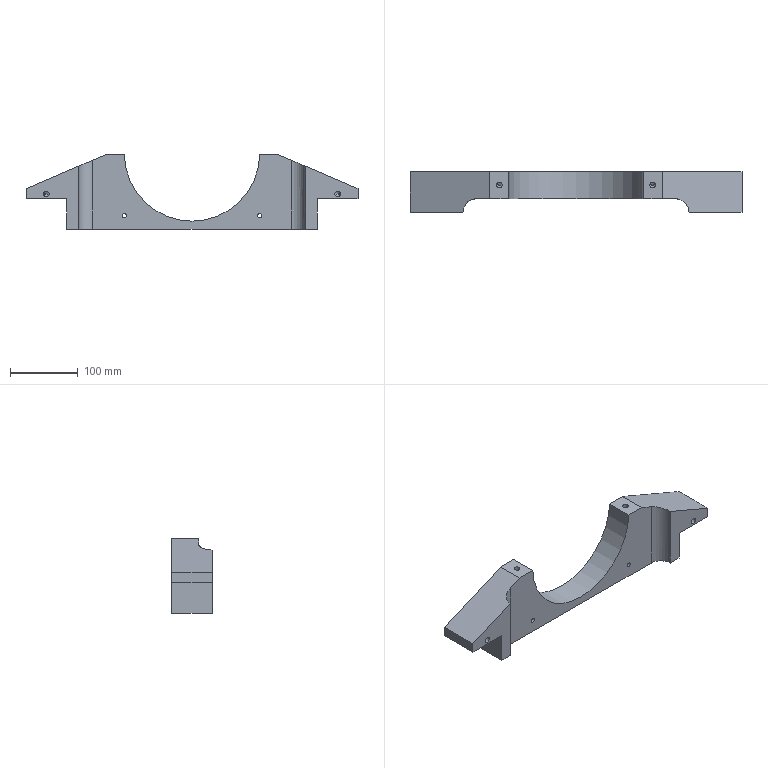Part | NX | features BREP 1 | 1 solid | 44 faces | box 490 x 60 x 110 mm | volume 1231742 mm3 | cylinder 19 | plane 17 | cone 8 | commonest cylinder face diameters 8.376 x8 6.4 x4 11.2 x4 40 x2 200 x1
STEP:
#1=CARTESIAN_POINT('',(185.,20.,-111.215));
#2=VERTEX_POINT('',#1);
#3=CARTESIAN_POINT('',(185.,20.,-66.215));
#4=VERTEX_POINT('',#3);
#5=CARTESIAN_POINT('',(185.,20.,-111.215));
#6=DIRECTION('',(0.,0.,1.));
#7=VECTOR('',#6,1000.);
#8=LINE('',#5,#7);
#9=EDGE_CURVE('',#2,#4,#8,.T.);
#10=ORIENTED_EDGE('',*,*,#9,.T.);
#11=CARTESIAN_POINT('',(185.,-40.,-66.215));
#12=VERTEX_POINT('',#11);
#13=CARTESIAN_POINT('',(185.,-40.,-66.215));
#14=DIRECTION('',(0.,1.,0.));
#15=VECTOR('',#14,1000.);
#16=LINE('',#13,#15);
#17=EDGE_CURVE('',#12,#4,#16,.T.);
#18=ORIENTED_EDGE('',*,*,#17,.F.);
#19=CARTESIAN_POINT('',(185.,-40.,-111.215));
#20=VERTEX_POINT('',#19);
#21=CARTESIAN_POINT('',(185.,-40.,-66.215));
#22=DIRECTION('',(0.,0.,-1.));
#23=VECTOR('',#22,1000.);
#24=LINE('',#21,#23);
#25=EDGE_CURVE('',#12,#20,#24,.T.);
#26=ORIENTED_EDGE('',*,*,#25,.T.);
#27=CARTESIAN_POINT('',(185.,-40.,-111.215));
#28=DIRECTION('',(0.,1.,0.));
#29=VECTOR('',#28,1000.);
#30=LINE('',#27,#29);
#31=EDGE_CURVE('',#20,#2,#30,.T.);
#32=ORIENTED_EDGE('',*,*,#31,.T.);
#33=EDGE_LOOP('',(#10,#18,#26,#32));
#34=FACE_BOUND('',#33,.T.);
#35=CARTESIAN_POINT('',(185.,0.,-121.215));
#36=DIRECTION('',(-1.,0.,0.));
#37=DIRECTION('',(0.,0.,1.));
#38=AXIS2_PLACEMENT_3D('',#35,#36,#37);
#39=PLANE('',#38);
#40=ADVANCED_FACE('',(#34),#39,.F.);
#41=CARTESIAN_POINT('',(-146.78,-20.,-111.215));
#42=VERTEX_POINT('',#41);
#43=CARTESIAN_POINT('',(-166.78,-40.,-111.215));
#44=VERTEX_POINT('',#43);
#45=CARTESIAN_POINT('',(-146.78,-40.,-111.215));
#46=DIRECTION('',(0.,0.,1.));
#47=DIRECTION('',(0.,1.,0.));
#48=AXIS2_PLACEMENT_3D('',#45,#46,#47);
#49=CIRCLE('',#48,20.);
#50=EDGE_CURVE('',#42,#44,#49,.T.);
#51=ORIENTED_EDGE('',*,*,#50,.T.);
#52=CARTESIAN_POINT('',(-185.,-40.,-111.215));
#53=VERTEX_POINT('',#52);
#54=CARTESIAN_POINT('',(-166.78,-40.,-111.215));
#55=DIRECTION('',(-1.,0.,0.));
#56=VECTOR('',#55,1000.);
#57=LINE('',#54,#56);
#58=EDGE_CURVE('',#44,#53,#57,.T.);
#59=ORIENTED_EDGE('',*,*,#58,.T.);
#60=CARTESIAN_POINT('',(-185.,20.,-111.215));
#61=VERTEX_POINT('',#60);
#62=CARTESIAN_POINT('',(-185.,-40.,-111.215));
#63=DIRECTION('',(0.,1.,0.));
#64=VECTOR('',#63,1000.);
#65=LINE('',#62,#64);
#66=EDGE_CURVE('',#53,#61,#65,.T.);
#67=ORIENTED_EDGE('',*,*,#66,.T.);
#68=CARTESIAN_POINT('',(185.,20.,-111.215));
#69=DIRECTION('',(-1.,0.,0.));
#70=VECTOR('',#69,1000.);
#71=LINE('',#68,#70);
#72=EDGE_CURVE('',#2,#61,#71,.T.);
#73=ORIENTED_EDGE('',*,*,#72,.F.);
#74=ORIENTED_EDGE('',*,*,#31,.F.);
#75=CARTESIAN_POINT('',(166.78,-40.,-111.215));
#76=VERTEX_POINT('',#75);
#77=CARTESIAN_POINT('',(166.78,-40.,-111.215));
#78=DIRECTION('',(1.,0.,0.));
#79=VECTOR('',#78,1000.);
#80=LINE('',#77,#79);
#81=EDGE_CURVE('',#76,#20,#80,.T.);
#82=ORIENTED_EDGE('',*,*,#81,.F.);
#83=CARTESIAN_POINT('',(146.78,-20.,-111.215));
#84=VERTEX_POINT('',#83);
#85=CARTESIAN_POINT('',(146.78,-40.,-111.215));
#86=DIRECTION('',(0.,0.,1.));
#87=DIRECTION('',(1.,0.,0.));
#88=AXIS2_PLACEMENT_3D('',#85,#86,#87);
#89=CIRCLE('',#88,20.);
#90=EDGE_CURVE('',#76,#84,#89,.T.);
#91=ORIENTED_EDGE('',*,*,#90,.T.);
#92=CARTESIAN_POINT('',(-146.78,-20.,-111.215));
#93=DIRECTION('',(1.,0.,0.));
#94=VECTOR('',#93,1000.);
#95=LINE('',#92,#94);
#96=EDGE_CURVE('',#42,#84,#95,.T.);
#97=ORIENTED_EDGE('',*,*,#96,.F.);
#98=EDGE_LOOP('',(#51,#59,#67,#73,#74,#82,#91,#97));
#99=FACE_BOUND('',#98,.T.);
#100=CARTESIAN_POINT('',(0.,0.,-111.215));
#101=DIRECTION('',(0.,0.,-1.));
#102=DIRECTION('',(0.,-1.,0.));
#103=AXIS2_PLACEMENT_3D('',#100,#101,#102);
#104=PLANE('',#103);
#105=ADVANCED_FACE('',(#99),#104,.T.);
#106=CARTESIAN_POINT('',(146.78,-20.,-9.42));
#107=VERTEX_POINT('',#106);
#108=CARTESIAN_POINT('',(146.78,-20.,-9.42));
#109=DIRECTION('',(0.,0.,-1.));
#110=VECTOR('',#109,1000.);
#111=LINE('',#108,#110);
#112=EDGE_CURVE('',#107,#84,#111,.T.);
#113=ORIENTED_EDGE('',*,*,#112,.F.);
#114=CARTESIAN_POINT('',(127.5,-20.,-1.215));
#115=VERTEX_POINT('',#114);
#116=CARTESIAN_POINT('',(146.78,-20.,-9.42));
#117=DIRECTION('',(-0.9202,0.,0.3916));
#118=VECTOR('',#117,1000.);
#119=LINE('',#116,#118);
#120=EDGE_CURVE('',#107,#115,#119,.T.);
#121=ORIENTED_EDGE('',*,*,#120,.T.);
#122=CARTESIAN_POINT('',(99.98,-20.,-1.215));
#123=VERTEX_POINT('',#122);
#124=CARTESIAN_POINT('',(127.5,-20.,-1.215));
#125=DIRECTION('',(-1.,0.,0.));
#126=VECTOR('',#125,1000.);
#127=LINE('',#124,#126);
#128=EDGE_CURVE('',#115,#123,#127,.T.);
#129=ORIENTED_EDGE('',*,*,#128,.T.);
#130=CARTESIAN_POINT('',(-99.98,-20.,-1.215));
#131=VERTEX_POINT('',#130);
#132=CARTESIAN_POINT('',(0.,-20.,0.7847));
#133=DIRECTION('',(0.,1.,0.));
#134=DIRECTION('',(0.9998,0.,-0.02));
#135=AXIS2_PLACEMENT_3D('',#132,#133,#134);
#136=CIRCLE('',#135,100.);
#137=EDGE_CURVE('',#123,#131,#136,.T.);
#138=ORIENTED_EDGE('',*,*,#137,.T.);
#139=CARTESIAN_POINT('',(-127.5,-20.,-1.215));
#140=VERTEX_POINT('',#139);
#141=CARTESIAN_POINT('',(-99.98,-20.,-1.215));
#142=DIRECTION('',(-1.,0.,0.));
#143=VECTOR('',#142,1000.);
#144=LINE('',#141,#143);
#145=EDGE_CURVE('',#131,#140,#144,.T.);
#146=ORIENTED_EDGE('',*,*,#145,.T.);
#147=CARTESIAN_POINT('',(-146.78,-20.,-9.42));
#148=VERTEX_POINT('',#147);
#149=CARTESIAN_POINT('',(-127.5,-20.,-1.215));
#150=DIRECTION('',(-0.9202,0.,-0.3916));
#151=VECTOR('',#150,1000.);
#152=LINE('',#149,#151);
#153=EDGE_CURVE('',#140,#148,#152,.T.);
#154=ORIENTED_EDGE('',*,*,#153,.T.);
#155=CARTESIAN_POINT('',(-146.78,-20.,-111.215));
#156=DIRECTION('',(0.,0.,1.));
#157=VECTOR('',#156,1000.);
#158=LINE('',#155,#157);
#159=EDGE_CURVE('',#42,#148,#158,.T.);
#160=ORIENTED_EDGE('',*,*,#159,.F.);
#161=ORIENTED_EDGE('',*,*,#96,.T.);
#162=EDGE_LOOP('',(#113,#121,#129,#138,#146,#154,#160,#161));
#163=FACE_BOUND('',#162,.T.);
#164=CARTESIAN_POINT('',(96.8,-20.,-91.215));
#165=VERTEX_POINT('',#164);
#166=CARTESIAN_POINT('',(103.2,-20.,-91.215));
#167=VERTEX_POINT('',#166);
#168=CARTESIAN_POINT('',(100.,-20.,-91.215));
#169=DIRECTION('',(0.,1.,0.));
#170=DIRECTION('',(-1.,0.,0.));
#171=AXIS2_PLACEMENT_3D('',#168,#169,#170);
#172=CIRCLE('',#171,3.2);
#173=EDGE_CURVE('',#165,#167,#172,.T.);
#174=ORIENTED_EDGE('',*,*,#173,.T.);
#175=CARTESIAN_POINT('',(100.,-20.,-91.215));
#176=DIRECTION('',(0.,1.,0.));
#177=DIRECTION('',(1.,0.,0.));
#178=AXIS2_PLACEMENT_3D('',#175,#176,#177);
#179=CIRCLE('',#178,3.2);
#180=EDGE_CURVE('',#167,#165,#179,.T.);
#181=ORIENTED_EDGE('',*,*,#180,.T.);
#182=EDGE_LOOP('',(#174,#181));
#183=FACE_BOUND('',#182,.T.);
#184=CARTESIAN_POINT('',(-96.8,-20.,-91.215));
#185=VERTEX_POINT('',#184);
#186=CARTESIAN_POINT('',(-103.2,-20.,-91.215));
#187=VERTEX_POINT('',#186);
#188=CARTESIAN_POINT('',(-100.,-20.,-91.215));
#189=DIRECTION('',(0.,1.,0.));
#190=DIRECTION('',(1.,0.,0.));
#191=AXIS2_PLACEMENT_3D('',#188,#189,#190);
#192=CIRCLE('',#191,3.2);
#193=EDGE_CURVE('',#185,#187,#192,.T.);
#194=ORIENTED_EDGE('',*,*,#193,.T.);
#195=CARTESIAN_POINT('',(-100.,-20.,-91.215));
#196=DIRECTION('',(0.,1.,0.));
#197=DIRECTION('',(-1.,0.,0.));
#198=AXIS2_PLACEMENT_3D('',#195,#196,#197);
#199=CIRCLE('',#198,3.2);
#200=EDGE_CURVE('',#187,#185,#199,.T.);
#201=ORIENTED_EDGE('',*,*,#200,.T.);
#202=EDGE_LOOP('',(#194,#201));
#203=FACE_BOUND('',#202,.T.);
#204=CARTESIAN_POINT('',(0.,-20.,0.));
#205=DIRECTION('',(0.,1.,0.));
#206=DIRECTION('',(1.,0.,0.));
#207=AXIS2_PLACEMENT_3D('',#204,#205,#206);
#208=PLANE('',#207);
#209=ADVANCED_FACE('',(#163,#183,#203),#208,.F.);
#210=CARTESIAN_POINT('',(-96.8,14.,-91.215));
#211=VERTEX_POINT('',#210);
#212=CARTESIAN_POINT('',(-103.2,14.,-91.215));
#213=VERTEX_POINT('',#212);
#214=CARTESIAN_POINT('',(-100.,14.,-91.215));
#215=DIRECTION('',(0.,-1.,0.));
#216=DIRECTION('',(1.,0.,0.));
#217=AXIS2_PLACEMENT_3D('',#214,#215,#216);
#218=CIRCLE('',#217,3.2);
#219=EDGE_CURVE('',#211,#213,#218,.T.);
#220=ORIENTED_EDGE('',*,*,#219,.F.);
#221=CARTESIAN_POINT('',(-96.8,14.,-91.215));
#222=DIRECTION('',(0.,-1.,0.));
#223=VECTOR('',#222,1000.);
#224=LINE('',#221,#223);
#225=EDGE_CURVE('',#185,#211,#224,.F.);
#226=ORIENTED_EDGE('',*,*,#225,.F.);
#227=ORIENTED_EDGE('',*,*,#200,.F.);
#228=CARTESIAN_POINT('',(-103.2,14.,-91.215));
#229=DIRECTION('',(0.,-1.,0.));
#230=VECTOR('',#229,1000.);
#231=LINE('',#228,#230);
#232=EDGE_CURVE('',#187,#213,#231,.F.);
#233=ORIENTED_EDGE('',*,*,#232,.T.);
#234=EDGE_LOOP('',(#220,#226,#227,#233));
#235=FACE_BOUND('',#234,.T.);
#236=CARTESIAN_POINT('',(-100.,20.,-91.215));
#237=DIRECTION('',(0.,1.,0.));
#238=DIRECTION('',(-1.,0.,0.));
#239=AXIS2_PLACEMENT_3D('',#236,#237,#238);
#240=CYLINDRICAL_SURFACE('',#239,3.2);
#241=ADVANCED_FACE('',(#235),#240,.F.);
#242=CARTESIAN_POINT('',(-100.,14.,-91.215));
#243=DIRECTION('',(0.,-1.,0.));
#244=DIRECTION('',(-1.,0.,0.));
#245=AXIS2_PLACEMENT_3D('',#242,#243,#244);
#246=CIRCLE('',#245,3.2);
#247=EDGE_CURVE('',#213,#211,#246,.T.);
#248=ORIENTED_EDGE('',*,*,#247,.F.);
#249=ORIENTED_EDGE('',*,*,#232,.F.);
#250=ORIENTED_EDGE('',*,*,#193,.F.);
#251=ORIENTED_EDGE('',*,*,#225,.T.);
#252=EDGE_LOOP('',(#248,#249,#250,#251));
#253=FACE_BOUND('',#252,.T.);
#254=CARTESIAN_POINT('',(-100.,20.,-91.215));
#255=DIRECTION('',(0.,1.,0.));
#256=DIRECTION('',(-1.,0.,0.));
#257=AXIS2_PLACEMENT_3D('',#254,#255,#256);
#258=CYLINDRICAL_SURFACE('',#257,3.2);
#259=ADVANCED_FACE('',(#253),#258,.F.);
#260=CARTESIAN_POINT('',(-105.6,14.,-91.215));
#261=VERTEX_POINT('',#260);
#262=CARTESIAN_POINT('',(-94.4,14.,-91.215));
#263=VERTEX_POINT('',#262);
#264=CARTESIAN_POINT('',(-100.,14.,-91.215));
#265=DIRECTION('',(0.,1.,0.));
#266=DIRECTION('',(-1.,0.,0.));
#267=AXIS2_PLACEMENT_3D('',#264,#265,#266);
#268=CIRCLE('',#267,5.6);
#269=EDGE_CURVE('',#261,#263,#268,.T.);
#270=ORIENTED_EDGE('',*,*,#269,.T.);
#271=CARTESIAN_POINT('',(-100.,14.,-91.215));
#272=DIRECTION('',(0.,1.,0.));
#273=DIRECTION('',(1.,0.,0.));
#274=AXIS2_PLACEMENT_3D('',#271,#272,#273);
#275=CIRCLE('',#274,5.6);
#276=EDGE_CURVE('',#263,#261,#275,.T.);
#277=ORIENTED_EDGE('',*,*,#276,.T.);
#278=EDGE_LOOP('',(#270,#277));
#279=FACE_BOUND('',#278,.T.);
#280=ORIENTED_EDGE('',*,*,#247,.T.);
#281=ORIENTED_EDGE('',*,*,#219,.T.);
#282=EDGE_LOOP('',(#280,#281));
#283=FACE_BOUND('',#282,.T.);
#284=CARTESIAN_POINT('',(103.2,14.,-91.215));
#285=DIRECTION('',(0.,-1.,0.));
#286=DIRECTION('',(0.,0.,-1.));
#287=AXIS2_PLACEMENT_3D('',#284,#285,#286);
#288=PLANE('',#287);
#289=ADVANCED_FACE('',(#279,#283),#288,.F.);
#290=ORIENTED_EDGE('',*,*,#276,.F.);
#291=CARTESIAN_POINT('',(-94.4,20.,-91.215));
#292=VERTEX_POINT('',#291);
#293=CARTESIAN_POINT('',(-94.4,20.,-91.215));
#294=DIRECTION('',(0.,-1.,0.));
#295=VECTOR('',#294,1000.);
#296=LINE('',#293,#295);
#297=EDGE_CURVE('',#263,#292,#296,.F.);
#298=ORIENTED_EDGE('',*,*,#297,.T.);
#299=CARTESIAN_POINT('',(-105.6,20.,-91.215));
#300=VERTEX_POINT('',#299);
#301=CARTESIAN_POINT('',(-100.,20.,-91.215));
#302=DIRECTION('',(0.,-1.,0.));
#303=DIRECTION('',(-1.,0.,0.));
#304=AXIS2_PLACEMENT_3D('',#301,#302,#303);
#305=CIRCLE('',#304,5.6);
#306=EDGE_CURVE('',#300,#292,#305,.T.);
#307=ORIENTED_EDGE('',*,*,#306,.F.);
#308=CARTESIAN_POINT('',(-105.6,20.,-91.215));
#309=DIRECTION('',(0.,-1.,0.));
#310=VECTOR('',#309,1000.);
#311=LINE('',#308,#310);
#312=EDGE_CURVE('',#261,#300,#311,.F.);
#313=ORIENTED_EDGE('',*,*,#312,.F.);
#314=EDGE_LOOP('',(#290,#298,#307,#313));
#315=FACE_BOUND('',#314,.T.);
#316=CARTESIAN_POINT('',(-100.,20.,-91.215));
#317=DIRECTION('',(0.,1.,0.));
#318=DIRECTION('',(-1.,0.,0.));
#319=AXIS2_PLACEMENT_3D('',#316,#317,#318);
#320=CYLINDRICAL_SURFACE('',#319,5.6);
#321=ADVANCED_FACE('',(#315),#320,.F.);
#322=ORIENTED_EDGE('',*,*,#269,.F.);
#323=ORIENTED_EDGE('',*,*,#312,.T.);
#324=CARTESIAN_POINT('',(-100.,20.,-91.215));
#325=DIRECTION('',(0.,-1.,0.));
#326=DIRECTION('',(1.,0.,0.));
#327=AXIS2_PLACEMENT_3D('',#324,#325,#326);
#328=CIRCLE('',#327,5.6);
#329=EDGE_CURVE('',#292,#300,#328,.T.);
#330=ORIENTED_EDGE('',*,*,#329,.F.);
#331=ORIENTED_EDGE('',*,*,#297,.F.);
#332=EDGE_LOOP('',(#322,#323,#330,#331));
#333=FACE_BOUND('',#332,.T.);
#334=CARTESIAN_POINT('',(-100.,20.,-91.215));
#335=DIRECTION('',(0.,1.,0.));
#336=DIRECTION('',(-1.,0.,0.));
#337=AXIS2_PLACEMENT_3D('',#334,#335,#336);
#338=CYLINDRICAL_SURFACE('',#337,5.6);
#339=ADVANCED_FACE('',(#333),#338,.F.);
#340=CARTESIAN_POINT('',(-185.,20.,-66.215));
#341=VERTEX_POINT('',#340);
#342=CARTESIAN_POINT('',(-185.,20.,-66.215));
#343=DIRECTION('',(0.,0.,-1.));
#344=VECTOR('',#343,1000.);
#345=LINE('',#342,#344);
#346=EDGE_CURVE('',#341,#61,#345,.T.);
#347=ORIENTED_EDGE('',*,*,#346,.F.);
#348=CARTESIAN_POINT('',(-245.,20.,-66.215));
#349=VERTEX_POINT('',#348);
#350=CARTESIAN_POINT('',(-245.,20.,-66.215));
#351=DIRECTION('',(1.,0.,0.));
#352=VECTOR('',#351,1000.);
#353=LINE('',#350,#352);
#354=EDGE_CURVE('',#349,#341,#353,.T.);
#355=ORIENTED_EDGE('',*,*,#354,.F.);
#356=CARTESIAN_POINT('',(-245.,20.,-51.215));
#357=VERTEX_POINT('',#356);
#358=CARTESIAN_POINT('',(-245.,20.,-51.215));
#359=DIRECTION('',(0.,0.,-1.));
#360=VECTOR('',#359,1000.);
#361=LINE('',#358,#360);
#362=EDGE_CURVE('',#357,#349,#361,.T.);
#363=ORIENTED_EDGE('',*,*,#362,.F.);
#364=CARTESIAN_POINT('',(-127.5,20.,-1.215));
#365=VERTEX_POINT('',#364);
#366=CARTESIAN_POINT('',(-245.,20.,-51.215));
#367=DIRECTION('',(0.9202,0.,0.3916));
#368=VECTOR('',#367,1000.);
#369=LINE('',#366,#368);
#370=EDGE_CURVE('',#357,#365,#369,.T.);
#371=ORIENTED_EDGE('',*,*,#370,.T.);
#372=CARTESIAN_POINT('',(-99.98,20.,-1.215));
#373=VERTEX_POINT('',#372);
#374=CARTESIAN_POINT('',(-99.98,20.,-1.215));
#375=DIRECTION('',(-1.,0.,0.));
#376=VECTOR('',#375,1000.);
#377=LINE('',#374,#376);
#378=EDGE_CURVE('',#373,#365,#377,.T.);
#379=ORIENTED_EDGE('',*,*,#378,.F.);
#380=CARTESIAN_POINT('',(99.98,20.,-1.215));
#381=VERTEX_POINT('',#380);
#382=CARTESIAN_POINT('',(0.,20.,0.7847));
#383=DIRECTION('',(0.,-1.,0.));
#384=DIRECTION('',(-0.9998,0.,-0.02));
#385=AXIS2_PLACEMENT_3D('',#382,#383,#384);
#386=CIRCLE('',#385,100.);
#387=EDGE_CURVE('',#373,#381,#386,.T.);
#388=ORIENTED_EDGE('',*,*,#387,.T.);
#389=CARTESIAN_POINT('',(127.5,20.,-1.215));
#390=VERTEX_POINT('',#389);
#391=CARTESIAN_POINT('',(127.5,20.,-1.215));
#392=DIRECTION('',(-1.,0.,0.));
#393=VECTOR('',#392,1000.);
#394=LINE('',#391,#393);
#395=EDGE_CURVE('',#390,#381,#394,.T.);
#396=ORIENTED_EDGE('',*,*,#395,.F.);
#397=CARTESIAN_POINT('',(245.,20.,-51.215));
#398=VERTEX_POINT('',#397);
#399=CARTESIAN_POINT('',(127.5,20.,-1.215));
#400=DIRECTION('',(0.9202,0.,-0.3916));
#401=VECTOR('',#400,1000.);
#402=LINE('',#399,#401);
#403=EDGE_CURVE('',#390,#398,#402,.T.);
#404=ORIENTED_EDGE('',*,*,#403,.T.);
#405=CARTESIAN_POINT('',(245.,20.,-66.215));
#406=VERTEX_POINT('',#405);
#407=CARTESIAN_POINT('',(245.,20.,-66.215));
#408=DIRECTION('',(0.,0.,1.));
#409=VECTOR('',#408,1000.);
#410=LINE('',#407,#409);
#411=EDGE_CURVE('',#406,#398,#410,.T.);
#412=ORIENTED_EDGE('',*,*,#411,.F.);
#413=CARTESIAN_POINT('',(185.,20.,-66.215));
#414=DIRECTION('',(1.,0.,0.));
#415=VECTOR('',#414,1000.);
#416=LINE('',#413,#415);
#417=EDGE_CURVE('',#4,#406,#416,.T.);
#418=ORIENTED_EDGE('',*,*,#417,.F.);
#419=ORIENTED_EDGE('',*,*,#9,.F.);
#420=ORIENTED_EDGE('',*,*,#72,.T.);
#421=EDGE_LOOP('',(#347,#355,#363,#371,#379,#388,#396,#404,#412,#418,#419,#420));
#422=FACE_BOUND('',#421,.T.);
#423=CARTESIAN_POINT('',(94.4,20.,-91.215));
#424=VERTEX_POINT('',#423);
#425=CARTESIAN_POINT('',(105.6,20.,-91.215));
#426=VERTEX_POINT('',#425);
#427=CARTESIAN_POINT('',(100.,20.,-91.215));
#428=DIRECTION('',(0.,-1.,0.));
#429=DIRECTION('',(-1.,0.,0.));
#430=AXIS2_PLACEMENT_3D('',#427,#428,#429);
#431=CIRCLE('',#430,5.6);
#432=EDGE_CURVE('',#424,#426,#431,.T.);
#433=ORIENTED_EDGE('',*,*,#432,.T.);
#434=CARTESIAN_POINT('',(100.,20.,-91.215));
#435=DIRECTION('',(0.,-1.,0.));
#436=DIRECTION('',(1.,0.,0.));
#437=AXIS2_PLACEMENT_3D('',#434,#435,#436);
#438=CIRCLE('',#437,5.6);
#439=EDGE_CURVE('',#426,#424,#438,.T.);
#440=ORIENTED_EDGE('',*,*,#439,.T.);
#441=EDGE_LOOP('',(#433,#440));
#442=FACE_BOUND('',#441,.T.);
#443=ORIENTED_EDGE('',*,*,#329,.T.);
#444=ORIENTED_EDGE('',*,*,#306,.T.);
#445=EDGE_LOOP('',(#443,#444));
#446=FACE_BOUND('',#445,.T.);
#447=CARTESIAN_POINT('',(0.,20.,0.));
#448=DIRECTION('',(0.,1.,0.));
#449=DIRECTION('',(1.,0.,0.));
#450=AXIS2_PLACEMENT_3D('',#447,#448,#449);
#451=PLANE('',#450);
#452=ADVANCED_FACE('',(#422,#442,#446),#451,.T.);
#453=CARTESIAN_POINT('',(105.6,14.,-91.215));
#454=VERTEX_POINT('',#453);
#455=CARTESIAN_POINT('',(105.6,20.,-91.215));
#456=DIRECTION('',(0.,-1.,0.));
#457=VECTOR('',#456,1000.);
#458=LINE('',#455,#457);
#459=EDGE_CURVE('',#454,#426,#458,.F.);
#460=ORIENTED_EDGE('',*,*,#459,.F.);
#461=CARTESIAN_POINT('',(94.4,14.,-91.215));
#462=VERTEX_POINT('',#461);
#463=CARTESIAN_POINT('',(100.,14.,-91.215));
#464=DIRECTION('',(0.,1.,0.));
#465=DIRECTION('',(-1.,0.,0.));
#466=AXIS2_PLACEMENT_3D('',#463,#464,#465);
#467=CIRCLE('',#466,5.6);
#468=EDGE_CURVE('',#462,#454,#467,.T.);
#469=ORIENTED_EDGE('',*,*,#468,.F.);
#470=CARTESIAN_POINT('',(94.4,20.,-91.215));
#471=DIRECTION('',(0.,-1.,0.));
#472=VECTOR('',#471,1000.);
#473=LINE('',#470,#472);
#474=EDGE_CURVE('',#462,#424,#473,.F.);
#475=ORIENTED_EDGE('',*,*,#474,.T.);
#476=ORIENTED_EDGE('',*,*,#439,.F.);
#477=EDGE_LOOP('',(#460,#469,#475,#476));
#478=FACE_BOUND('',#477,.T.);
#479=CARTESIAN_POINT('',(100.,20.,-91.215));
#480=DIRECTION('',(0.,-1.,0.));
#481=DIRECTION('',(1.,0.,0.));
#482=AXIS2_PLACEMENT_3D('',#479,#480,#481);
#483=CYLINDRICAL_SURFACE('',#482,5.6);
#484=ADVANCED_FACE('',(#478),#483,.F.);
#485=ORIENTED_EDGE('',*,*,#474,.F.);
#486=CARTESIAN_POINT('',(100.,14.,-91.215));
#487=DIRECTION('',(0.,1.,0.));
#488=DIRECTION('',(1.,0.,0.));
#489=AXIS2_PLACEMENT_3D('',#486,#487,#488);
#490=CIRCLE('',#489,5.6);
#491=EDGE_CURVE('',#454,#462,#490,.T.);
#492=ORIENTED_EDGE('',*,*,#491,.F.);
#493=ORIENTED_EDGE('',*,*,#459,.T.);
#494=ORIENTED_EDGE('',*,*,#432,.F.);
#495=EDGE_LOOP('',(#485,#492,#493,#494));
#496=FACE_BOUND('',#495,.T.);
#497=CARTESIAN_POINT('',(100.,20.,-91.215));
#498=DIRECTION('',(0.,-1.,0.));
#499=DIRECTION('',(1.,0.,0.));
#500=AXIS2_PLACEMENT_3D('',#497,#498,#499);
#501=CYLINDRICAL_SURFACE('',#500,5.6);
#502=ADVANCED_FACE('',(#496),#501,.F.);
#503=ORIENTED_EDGE('',*,*,#491,.T.);
#504=ORIENTED_EDGE('',*,*,#468,.T.);
#505=EDGE_LOOP('',(#503,#504));
#506=FACE_BOUND('',#505,.T.);
#507=CARTESIAN_POINT('',(103.2,14.,-91.215));
#508=VERTEX_POINT('',#507);
#509=CARTESIAN_POINT('',(96.8,14.,-91.215));
#510=VERTEX_POINT('',#509);
#511=CARTESIAN_POINT('',(100.,14.,-91.215));
#512=DIRECTION('',(0.,-1.,0.));
#513=DIRECTION('',(1.,0.,0.));
#514=AXIS2_PLACEMENT_3D('',#511,#512,#513);
#515=CIRCLE('',#514,3.2);
#516=EDGE_CURVE('',#508,#510,#515,.T.);
#517=ORIENTED_EDGE('',*,*,#516,.T.);
#518=CARTESIAN_POINT('',(100.,14.,-91.215));
#519=DIRECTION('',(0.,-1.,0.));
#520=DIRECTION('',(-1.,0.,0.));
#521=AXIS2_PLACEMENT_3D('',#518,#519,#520);
#522=CIRCLE('',#521,3.2);
#523=EDGE_CURVE('',#510,#508,#522,.T.);
#524=ORIENTED_EDGE('',*,*,#523,.T.);
#525=EDGE_LOOP('',(#517,#524));
#526=FACE_BOUND('',#525,.T.);
#527=CARTESIAN_POINT('',(103.2,14.,-91.215));
#528=DIRECTION('',(0.,-1.,0.));
#529=DIRECTION('',(0.,0.,-1.));
#530=AXIS2_PLACEMENT_3D('',#527,#528,#529);
#531=PLANE('',#530);
#532=ADVANCED_FACE('',(#506,#526),#531,.F.);
#533=CARTESIAN_POINT('',(103.2,14.,-91.215));
#534=DIRECTION('',(0.,-1.,0.));
#535=VECTOR('',#534,1000.);
#536=LINE('',#533,#535);
#537=EDGE_CURVE('',#167,#508,#536,.F.);
#538=ORIENTED_EDGE('',*,*,#537,.T.);
#539=ORIENTED_EDGE('',*,*,#523,.F.);
#540=CARTESIAN_POINT('',(96.8,14.,-91.215));
#541=DIRECTION('',(0.,-1.,0.));
#542=VECTOR('',#541,1000.);
#543=LINE('',#540,#542);
#544=EDGE_CURVE('',#165,#510,#543,.F.);
#545=ORIENTED_EDGE('',*,*,#544,.F.);
#546=ORIENTED_EDGE('',*,*,#180,.F.);
#547=EDGE_LOOP('',(#538,#539,#545,#546));
#548=FACE_BOUND('',#547,.T.);
#549=CARTESIAN_POINT('',(100.,20.,-91.215));
#550=DIRECTION('',(0.,-1.,0.));
#551=DIRECTION('',(1.,0.,0.));
#552=AXIS2_PLACEMENT_3D('',#549,#550,#551);
#553=CYLINDRICAL_SURFACE('',#552,3.2);
#554=ADVANCED_FACE('',(#548),#553,.F.);
#555=ORIENTED_EDGE('',*,*,#544,.T.);
#556=ORIENTED_EDGE('',*,*,#516,.F.);
#557=ORIENTED_EDGE('',*,*,#537,.F.);
#558=ORIENTED_EDGE('',*,*,#173,.F.);
#559=EDGE_LOOP('',(#555,#556,#557,#558));
#560=FACE_BOUND('',#559,.T.);
#561=CARTESIAN_POINT('',(100.,20.,-91.215));
#562=DIRECTION('',(0.,-1.,0.));
#563=DIRECTION('',(1.,0.,0.));
#564=AXIS2_PLACEMENT_3D('',#561,#562,#563);
#565=CYLINDRICAL_SURFACE('',#564,3.2);
#566=ADVANCED_FACE('',(#560),#565,.F.);
#567=CARTESIAN_POINT('',(245.,-40.,-66.215));
#568=VERTEX_POINT('',#567);
#569=CARTESIAN_POINT('',(185.,-40.,-66.215));
#570=DIRECTION('',(1.,0.,0.));
#571=VECTOR('',#570,1000.);
#572=LINE('',#569,#571);
#573=EDGE_CURVE('',#12,#568,#572,.T.);
#574=ORIENTED_EDGE('',*,*,#573,.F.);
#575=ORIENTED_EDGE('',*,*,#17,.T.);
#576=ORIENTED_EDGE('',*,*,#417,.T.);
#577=CARTESIAN_POINT('',(245.,-40.,-66.215));
#578=DIRECTION('',(0.,1.,0.));
#579=VECTOR('',#578,1000.);
#580=LINE('',#577,#579);
#581=EDGE_CURVE('',#568,#406,#580,.T.);
#582=ORIENTED_EDGE('',*,*,#581,.F.);
#583=EDGE_LOOP('',(#574,#575,#576,#582));
#584=FACE_BOUND('',#583,.T.);
#585=CARTESIAN_POINT('',(185.,0.,-66.215));
#586=DIRECTION('',(0.,0.,1.));
#587=DIRECTION('',(1.,0.,0.));
#588=AXIS2_PLACEMENT_3D('',#585,#586,#587);
#589=PLANE('',#588);
#590=ADVANCED_FACE('',(#584),#589,.F.);
#591=ORIENTED_EDGE('',*,*,#411,.T.);
#592=CARTESIAN_POINT('',(245.,-40.,-51.215));
#593=VERTEX_POINT('',#592);
#594=CARTESIAN_POINT('',(245.,-40.,-51.215));
#595=DIRECTION('',(0.,1.,0.));
#596=VECTOR('',#595,1000.);
#597=LINE('',#594,#596);
#598=EDGE_CURVE('',#593,#398,#597,.T.);
#599=ORIENTED_EDGE('',*,*,#598,.F.);
#600=CARTESIAN_POINT('',(245.,-40.,-51.215));
#601=DIRECTION('',(0.,0.,-1.));
#602=VECTOR('',#601,1000.);
#603=LINE('',#600,#602);
#604=EDGE_CURVE('',#593,#568,#603,.T.);
#605=ORIENTED_EDGE('',*,*,#604,.T.);
#606=ORIENTED_EDGE('',*,*,#581,.T.);
#607=EDGE_LOOP('',(#591,#599,#605,#606));
#608=FACE_BOUND('',#607,.T.);
#609=CARTESIAN_POINT('',(245.,0.,-51.215));
#610=DIRECTION('',(1.,0.,0.));
#611=DIRECTION('',(0.,1.,0.));
#612=AXIS2_PLACEMENT_3D('',#609,#610,#611);
#613=PLANE('',#612);
#614=ADVANCED_FACE('',(#608),#613,.T.);
#615=ORIENTED_EDGE('',*,*,#25,.F.);
#616=ORIENTED_EDGE('',*,*,#573,.T.);
#617=ORIENTED_EDGE('',*,*,#604,.F.);
#618=CARTESIAN_POINT('',(166.78,-40.,-17.93));
#619=VERTEX_POINT('',#618);
#620=CARTESIAN_POINT('',(245.,-40.,-51.215));
#621=DIRECTION('',(-0.9202,0.,0.3916));
#622=VECTOR('',#621,1000.);
#623=LINE('',#620,#622);
#624=EDGE_CURVE('',#593,#619,#623,.T.);
#625=ORIENTED_EDGE('',*,*,#624,.T.);
#626=CARTESIAN_POINT('',(166.78,-40.,-111.215));
#627=DIRECTION('',(0.,0.,1.));
#628=VECTOR('',#627,1000.);
#629=LINE('',#626,#628);
#630=EDGE_CURVE('',#76,#619,#629,.T.);
#631=ORIENTED_EDGE('',*,*,#630,.F.);
#632=ORIENTED_EDGE('',*,*,#81,.T.);
#633=EDGE_LOOP('',(#615,#616,#617,#625,#631,#632));
#634=FACE_BOUND('',#633,.T.);
#635=CARTESIAN_POINT('',(219.188,-40.,-59.215));
#636=VERTEX_POINT('',#635);
#637=CARTESIAN_POINT('',(210.812,-40.,-59.215));
#638=VERTEX_POINT('',#637);
#639=CARTESIAN_POINT('',(215.,-40.,-59.215));
#640=DIRECTION('',(0.,1.,0.));
#641=DIRECTION('',(1.,0.,0.));
#642=AXIS2_PLACEMENT_3D('',#639,#640,#641);
#643=CIRCLE('',#642,4.188);
#644=EDGE_CURVE('',#636,#638,#643,.T.);
#645=ORIENTED_EDGE('',*,*,#644,.T.);
#646=CARTESIAN_POINT('',(215.,-40.,-59.215));
#647=DIRECTION('',(0.,1.,0.));
#648=DIRECTION('',(-1.,0.,0.));
#649=AXIS2_PLACEMENT_3D('',#646,#647,#648);
#650=CIRCLE('',#649,4.188);
#651=EDGE_CURVE('',#638,#636,#650,.T.);
#652=ORIENTED_EDGE('',*,*,#651,.T.);
#653=EDGE_LOOP('',(#645,#652));
#654=FACE_BOUND('',#653,.T.);
#655=CARTESIAN_POINT('',(245.,-40.,-121.215));
#656=DIRECTION('',(0.,1.,0.));
#657=DIRECTION('',(1.,0.,0.));
#658=AXIS2_PLACEMENT_3D('',#655,#656,#657);
#659=PLANE('',#658);
#660=ADVANCED_FACE('',(#634,#654),#659,.F.);
#661=CARTESIAN_POINT('',(210.812,-10.,-59.215));
#662=VERTEX_POINT('',#661);
#663=CARTESIAN_POINT('',(210.812,-40.,-59.215));
#664=DIRECTION('',(0.,1.,0.));
#665=VECTOR('',#664,1000.);
#666=LINE('',#663,#665);
#667=EDGE_CURVE('',#638,#662,#666,.T.);
#668=ORIENTED_EDGE('',*,*,#667,.T.);
#669=CARTESIAN_POINT('',(219.188,-10.,-59.215));
#670=VERTEX_POINT('',#669);
#671=CARTESIAN_POINT('',(215.,-10.,-59.215));
#672=DIRECTION('',(0.,-1.,0.));
#673=DIRECTION('',(1.,0.,0.));
#674=AXIS2_PLACEMENT_3D('',#671,#672,#673);
#675=CIRCLE('',#674,4.188);
#676=EDGE_CURVE('',#670,#662,#675,.T.);
#677=ORIENTED_EDGE('',*,*,#676,.F.);
#678=CARTESIAN_POINT('',(219.188,-40.,-59.215));
#679=DIRECTION('',(0.,1.,0.));
#680=VECTOR('',#679,1000.);
#681=LINE('',#678,#680);
#682=EDGE_CURVE('',#636,#670,#681,.T.);
#683=ORIENTED_EDGE('',*,*,#682,.F.);
#684=ORIENTED_EDGE('',*,*,#651,.F.);
#685=EDGE_LOOP('',(#668,#677,#683,#684));
#686=FACE_BOUND('',#685,.T.);
#687=CARTESIAN_POINT('',(215.,-40.,-59.215));
#688=DIRECTION('',(0.,1.,0.));
#689=DIRECTION('',(1.,0.,0.));
#690=AXIS2_PLACEMENT_3D('',#687,#688,#689);
#691=CYLINDRICAL_SURFACE('',#690,4.188);
#692=ADVANCED_FACE('',(#686),#691,.F.);
#693=ORIENTED_EDGE('',*,*,#682,.T.);
#694=CARTESIAN_POINT('',(215.,-10.,-59.215));
#695=DIRECTION('',(0.,-1.,0.));
#696=DIRECTION('',(-1.,0.,0.));
#697=AXIS2_PLACEMENT_3D('',#694,#695,#696);
#698=CIRCLE('',#697,4.188);
#699=EDGE_CURVE('',#662,#670,#698,.T.);
#700=ORIENTED_EDGE('',*,*,#699,.F.);
#701=ORIENTED_EDGE('',*,*,#667,.F.);
#702=ORIENTED_EDGE('',*,*,#644,.F.);
#703=EDGE_LOOP('',(#693,#700,#701,#702));
#704=FACE_BOUND('',#703,.T.);
#705=CARTESIAN_POINT('',(215.,-40.,-59.215));
#706=DIRECTION('',(0.,1.,0.));
#707=DIRECTION('',(1.,0.,0.));
#708=AXIS2_PLACEMENT_3D('',#705,#706,#707);
#709=CYLINDRICAL_SURFACE('',#708,4.188);
#710=ADVANCED_FACE('',(#704),#709,.F.);
#711=ORIENTED_EDGE('',*,*,#699,.T.);
#712=CARTESIAN_POINT('',(215.,-7.582,-59.215));
#713=VERTEX_POINT('',#712);
#714=CARTESIAN_POINT('',(219.188,-10.,-59.215));
#715=DIRECTION('',(-0.866,0.5,0.));
#716=VECTOR('',#715,1000.);
#717=LINE('',#714,#716);
#718=EDGE_CURVE('',#713,#670,#717,.F.);
#719=ORIENTED_EDGE('',*,*,#718,.F.);
#720=CARTESIAN_POINT('',(210.812,-10.,-59.215));
#721=DIRECTION('',(0.866,0.5,0.));
#722=VECTOR('',#721,1000.);
#723=LINE('',#720,#722);
#724=EDGE_CURVE('',#713,#662,#723,.F.);
#725=ORIENTED_EDGE('',*,*,#724,.T.);
#726=EDGE_LOOP('',(#711,#719,#725));
#727=FACE_BOUND('',#726,.T.);
#728=CARTESIAN_POINT('',(215.,-8.943,-59.215));
#729=DIRECTION('',(0.,-1.,0.));
#730=DIRECTION('',(1.,0.,0.));
#731=AXIS2_PLACEMENT_3D('',#728,#729,#730);
#732=CONICAL_SURFACE('',#731,2.358,1.047);
#733=ADVANCED_FACE('',(#727),#732,.F.);
#734=ORIENTED_EDGE('',*,*,#676,.T.);
#735=ORIENTED_EDGE('',*,*,#724,.F.);
#736=ORIENTED_EDGE('',*,*,#718,.T.);
#737=EDGE_LOOP('',(#734,#735,#736));
#738=FACE_BOUND('',#737,.T.);
#739=CARTESIAN_POINT('',(215.,-8.943,-59.215));
#740=DIRECTION('',(0.,-1.,0.));
#741=DIRECTION('',(1.,0.,0.));
#742=AXIS2_PLACEMENT_3D('',#739,#740,#741);
#743=CONICAL_SURFACE('',#742,2.358,1.047);
#744=ADVANCED_FACE('',(#738),#743,.F.);
#745=ORIENTED_EDGE('',*,*,#630,.T.);
#746=CARTESIAN_POINT('',(146.78,-20.,-9.42));
#747=CARTESIAN_POINT('',(148.294,-20.,-10.064));
#748=CARTESIAN_POINT('',(150.513,-20.248,-11.008));
#749=CARTESIAN_POINT('',(152.996,-20.963,-12.065));
#750=CARTESIAN_POINT('',(154.228,-21.436,-12.589));
#751=CARTESIAN_POINT('',(154.903,-21.725,-12.876));
#752=CARTESIAN_POINT('',(155.469,-21.989,-13.117));
#753=CARTESIAN_POINT('',(155.788,-22.148,-13.253));
#754=CARTESIAN_POINT('',(156.291,-22.407,-13.467));
#755=CARTESIAN_POINT('',(157.115,-22.866,-13.817));
#756=CARTESIAN_POINT('',(158.265,-23.601,-14.307));
#757=CARTESIAN_POINT('',(159.33,-24.41,-14.76));
#758=CARTESIAN_POINT('',(160.168,-25.136,-15.117));
#759=CARTESIAN_POINT('',(160.709,-25.638,-15.347));
#760=CARTESIAN_POINT('',(161.489,-26.432,-15.679));
#761=CARTESIAN_POINT('',(162.371,-27.438,-16.054));
#762=CARTESIAN_POINT('',(163.4,-28.805,-16.492));
#763=CARTESIAN_POINT('',(164.442,-30.539,-16.935));
#764=CARTESIAN_POINT('',(165.626,-33.08,-17.439));
#765=CARTESIAN_POINT('',(166.523,-36.107,-17.821));
#766=CARTESIAN_POINT('',(166.78,-38.693,-17.93));
#767=CARTESIAN_POINT('',(166.78,-40.,-17.93));
#768=B_SPLINE_CURVE_WITH_KNOTS('',3,(#746,#747,#748,#749,#750,#751,#752,#753,#754,#755,#756,#757,#758,#759,#760,#761,#762,#763,#764,#765,#766,#767),.UNSPECIFIED.,.F.,.F.,(4,1,1,1,1,1,1,1,1,1,1,1,1,1,1,1,1,1,1,4),(0.,0.125,0.1875,0.2188,0.2344,0.25,0.2656,0.2812,0.3125,0.375,0.4375,0.4688,0.5,0.5312,0.5625,0.625,0.6875,0.75,0.875,1.),.UNSPECIFIED.);
#769=EDGE_CURVE('',#619,#107,#768,.F.);
#770=ORIENTED_EDGE('',*,*,#769,.T.);
#771=ORIENTED_EDGE('',*,*,#112,.T.);
#772=ORIENTED_EDGE('',*,*,#90,.F.);
#773=EDGE_LOOP('',(#745,#770,#771,#772));
#774=FACE_BOUND('',#773,.T.);
#775=CARTESIAN_POINT('',(146.78,-40.,-61.215));
#776=DIRECTION('',(0.,0.,1.));
#777=DIRECTION('',(1.,0.,0.));
#778=AXIS2_PLACEMENT_3D('',#775,#776,#777);
#779=CYLINDRICAL_SURFACE('',#778,20.);
#780=ADVANCED_FACE('',(#774),#779,.F.);
#781=ORIENTED_EDGE('',*,*,#598,.T.);
#782=ORIENTED_EDGE('',*,*,#403,.F.);
#783=CARTESIAN_POINT('',(127.5,20.,-1.215));
#784=DIRECTION('',(0.,-1.,0.));
#785=VECTOR('',#784,1000.);
#786=LINE('',#783,#785);
#787=EDGE_CURVE('',#390,#115,#786,.T.);
#788=ORIENTED_EDGE('',*,*,#787,.T.);
#789=ORIENTED_EDGE('',*,*,#120,.F.);
#790=ORIENTED_EDGE('',*,*,#769,.F.);
#791=ORIENTED_EDGE('',*,*,#624,.F.);
#792=EDGE_LOOP('',(#781,#782,#788,#789,#790,#791));
#793=FACE_BOUND('',#792,.T.);
#794=CARTESIAN_POINT('',(245.,0.,-51.215));
#795=DIRECTION('',(-0.3916,0.,-0.9202));
#796=DIRECTION('',(-0.9202,0.,0.3916));
#797=AXIS2_PLACEMENT_3D('',#794,#795,#796);
#798=PLANE('',#797);
#799=ADVANCED_FACE('',(#793),#798,.F.);
#800=ORIENTED_EDGE('',*,*,#128,.F.);
#801=ORIENTED_EDGE('',*,*,#787,.F.);
#802=ORIENTED_EDGE('',*,*,#395,.T.);
#803=CARTESIAN_POINT('',(99.98,-20.,-1.215));
#804=DIRECTION('',(0.,1.,0.));
#805=VECTOR('',#804,1000.);
#806=LINE('',#803,#805);
#807=EDGE_CURVE('',#123,#381,#806,.T.);
#808=ORIENTED_EDGE('',*,*,#807,.F.);
#809=EDGE_LOOP('',(#800,#801,#802,#808));
#810=FACE_BOUND('',#809,.T.);
#811=CARTESIAN_POINT('',(117.188,0.,-1.215));
#812=VERTEX_POINT('',#811);
#813=CARTESIAN_POINT('',(108.812,0.,-1.215));
#814=VERTEX_POINT('',#813);
#815=CARTESIAN_POINT('',(113.,0.,-1.215));
#816=DIRECTION('',(0.,0.,-1.));
#817=DIRECTION('',(1.,0.,0.));
#818=AXIS2_PLACEMENT_3D('',#815,#816,#817);
#819=CIRCLE('',#818,4.188);
#820=EDGE_CURVE('',#812,#814,#819,.T.);
#821=ORIENTED_EDGE('',*,*,#820,.T.);
#822=CARTESIAN_POINT('',(113.,0.,-1.215));
#823=DIRECTION('',(0.,0.,-1.));
#824=DIRECTION('',(-1.,0.,0.));
#825=AXIS2_PLACEMENT_3D('',#822,#823,#824);
#826=CIRCLE('',#825,4.188);
#827=EDGE_CURVE('',#814,#812,#826,.T.);
#828=ORIENTED_EDGE('',*,*,#827,.T.);
#829=EDGE_LOOP('',(#821,#828));
#830=FACE_BOUND('',#829,.T.);
#831=CARTESIAN_POINT('',(-99.98,0.,-1.215));
#832=DIRECTION('',(0.,0.,-1.));
#833=DIRECTION('',(0.,-1.,0.));
#834=AXIS2_PLACEMENT_3D('',#831,#832,#833);
#835=PLANE('',#834);
#836=ADVANCED_FACE('',(#810,#830),#835,.F.);
#837=ORIENTED_EDGE('',*,*,#137,.F.);
#838=ORIENTED_EDGE('',*,*,#807,.T.);
#839=ORIENTED_EDGE('',*,*,#387,.F.);
#840=CARTESIAN_POINT('',(-99.98,20.,-1.215));
#841=DIRECTION('',(0.,-1.,0.));
#842=VECTOR('',#841,1000.);
#843=LINE('',#840,#842);
#844=EDGE_CURVE('',#373,#131,#843,.T.);
#845=ORIENTED_EDGE('',*,*,#844,.T.);
#846=EDGE_LOOP('',(#837,#838,#839,#845));
#847=FACE_BOUND('',#846,.T.);
#848=CARTESIAN_POINT('',(0.,0.,0.7847));
#849=DIRECTION('',(0.,1.,0.));
#850=DIRECTION('',(0.9998,0.,-0.02));
#851=AXIS2_PLACEMENT_3D('',#848,#849,#850);
#852=CYLINDRICAL_SURFACE('',#851,100.);
#853=ADVANCED_FACE('',(#847),#852,.F.);
#854=ORIENTED_EDGE('',*,*,#145,.F.);
#855=ORIENTED_EDGE('',*,*,#844,.F.);
#856=ORIENTED_EDGE('',*,*,#378,.T.);
#857=CARTESIAN_POINT('',(-127.5,20.,-1.215));
#858=DIRECTION('',(0.,-1.,0.));
#859=VECTOR('',#858,1000.);
#860=LINE('',#857,#859);
#861=EDGE_CURVE('',#365,#140,#860,.T.);
#862=ORIENTED_EDGE('',*,*,#861,.T.);
#863=EDGE_LOOP('',(#854,#855,#856,#862));
#864=FACE_BOUND('',#863,.T.);
#865=CARTESIAN_POINT('',(-108.812,0.,-1.215));
#866=VERTEX_POINT('',#865);
#867=CARTESIAN_POINT('',(-117.188,0.,-1.215));
#868=VERTEX_POINT('',#867);
#869=CARTESIAN_POINT('',(-113.,0.,-1.215));
#870=DIRECTION('',(0.,0.,-1.));
#871=DIRECTION('',(1.,0.,0.));
#872=AXIS2_PLACEMENT_3D('',#869,#870,#871);
#873=CIRCLE('',#872,4.188);
#874=EDGE_CURVE('',#866,#868,#873,.T.);
#875=ORIENTED_EDGE('',*,*,#874,.T.);
#876=CARTESIAN_POINT('',(-113.,0.,-1.215));
#877=DIRECTION('',(0.,0.,-1.));
#878=DIRECTION('',(-1.,0.,0.));
#879=AXIS2_PLACEMENT_3D('',#876,#877,#878);
#880=CIRCLE('',#879,4.188);
#881=EDGE_CURVE('',#868,#866,#880,.T.);
#882=ORIENTED_EDGE('',*,*,#881,.T.);
#883=EDGE_LOOP('',(#875,#882));
#884=FACE_BOUND('',#883,.T.);
#885=CARTESIAN_POINT('',(-99.98,0.,-1.215));
#886=DIRECTION('',(0.,0.,-1.));
#887=DIRECTION('',(0.,-1.,0.));
#888=AXIS2_PLACEMENT_3D('',#885,#886,#887);
#889=PLANE('',#888);
#890=ADVANCED_FACE('',(#864,#884),#889,.F.);
#891=ORIENTED_EDGE('',*,*,#153,.F.);
#892=ORIENTED_EDGE('',*,*,#861,.F.);
#893=ORIENTED_EDGE('',*,*,#370,.F.);
#894=CARTESIAN_POINT('',(-245.,-40.,-51.215));
#895=VERTEX_POINT('',#894);
#896=CARTESIAN_POINT('',(-245.,20.,-51.215));
#897=DIRECTION('',(0.,-1.,0.));
#898=VECTOR('',#897,1000.);
#899=LINE('',#896,#898);
#900=EDGE_CURVE('',#357,#895,#899,.T.);
#901=ORIENTED_EDGE('',*,*,#900,.T.);
#902=CARTESIAN_POINT('',(-166.78,-40.,-17.93));
#903=VERTEX_POINT('',#902);
#904=CARTESIAN_POINT('',(-166.78,-40.,-17.93));
#905=DIRECTION('',(-0.9202,0.,-0.3916));
#906=VECTOR('',#905,1000.);
#907=LINE('',#904,#906);
#908=EDGE_CURVE('',#903,#895,#907,.T.);
#909=ORIENTED_EDGE('',*,*,#908,.F.);
#910=CARTESIAN_POINT('',(-166.78,-40.,-17.93));
#911=CARTESIAN_POINT('',(-166.78,-38.694,-17.93));
#912=CARTESIAN_POINT('',(-166.523,-36.109,-17.821));
#913=CARTESIAN_POINT('',(-165.625,-33.079,-17.439));
#914=CARTESIAN_POINT('',(-164.443,-30.54,-16.936));
#915=CARTESIAN_POINT('',(-163.401,-28.806,-16.492));
#916=CARTESIAN_POINT('',(-162.372,-27.439,-16.054));
#917=CARTESIAN_POINT('',(-161.489,-26.432,-15.679));
#918=CARTESIAN_POINT('',(-160.709,-25.638,-15.347));
#919=CARTESIAN_POINT('',(-160.169,-25.136,-15.117));
#920=CARTESIAN_POINT('',(-159.331,-24.41,-14.76));
#921=CARTESIAN_POINT('',(-158.266,-23.602,-14.307));
#922=CARTESIAN_POINT('',(-157.115,-22.867,-13.818));
#923=CARTESIAN_POINT('',(-156.291,-22.407,-13.467));
#924=CARTESIAN_POINT('',(-155.787,-22.148,-13.253));
#925=CARTESIAN_POINT('',(-155.468,-21.989,-13.117));
#926=CARTESIAN_POINT('',(-154.902,-21.725,-12.876));
#927=CARTESIAN_POINT('',(-154.228,-21.435,-12.589));
#928=CARTESIAN_POINT('',(-152.996,-20.963,-12.065));
#929=CARTESIAN_POINT('',(-150.513,-20.248,-11.008));
#930=CARTESIAN_POINT('',(-148.294,-20.,-10.064));
#931=CARTESIAN_POINT('',(-146.78,-20.,-9.42));
#932=B_SPLINE_CURVE_WITH_KNOTS('',3,(#910,#911,#912,#913,#914,#915,#916,#917,#918,#919,#920,#921,#922,#923,#924,#925,#926,#927,#928,#929,#930,#931),.UNSPECIFIED.,.F.,.F.,(4,1,1,1,1,1,1,1,1,1,1,1,1,1,1,1,1,1,1,4),(0.,0.125,0.25,0.3125,0.375,0.4375,0.4688,0.5,0.5312,0.5625,0.625,0.6875,0.7188,0.7344,0.75,0.7656,0.7812,0.8125,0.875,1.),.UNSPECIFIED.);
#933=EDGE_CURVE('',#148,#903,#932,.F.);
#934=ORIENTED_EDGE('',*,*,#933,.F.);
#935=EDGE_LOOP('',(#891,#892,#893,#901,#909,#934));
#936=FACE_BOUND('',#935,.T.);
#937=CARTESIAN_POINT('',(-245.,0.,-51.215));
#938=DIRECTION('',(-0.3916,0.,0.9202));
#939=DIRECTION('',(0.,1.,0.));
#940=AXIS2_PLACEMENT_3D('',#937,#938,#939);
#941=PLANE('',#940);
#942=ADVANCED_FACE('',(#936),#941,.T.);
#943=ORIENTED_EDGE('',*,*,#159,.T.);
#944=ORIENTED_EDGE('',*,*,#933,.T.);
#945=CARTESIAN_POINT('',(-166.78,-40.,-17.93));
#946=DIRECTION('',(0.,0.,-1.));
#947=VECTOR('',#946,1000.);
#948=LINE('',#945,#947);
#949=EDGE_CURVE('',#903,#44,#948,.T.);
#950=ORIENTED_EDGE('',*,*,#949,.T.);
#951=ORIENTED_EDGE('',*,*,#50,.F.);
#952=EDGE_LOOP('',(#943,#944,#950,#951));
#953=FACE_BOUND('',#952,.T.);
#954=CARTESIAN_POINT('',(-146.78,-40.,-61.215));
#955=DIRECTION('',(0.,0.,1.));
#956=DIRECTION('',(0.,1.,0.));
#957=AXIS2_PLACEMENT_3D('',#954,#955,#956);
#958=CYLINDRICAL_SURFACE('',#957,20.);
#959=ADVANCED_FACE('',(#953),#958,.F.);
#960=ORIENTED_EDGE('',*,*,#949,.F.);
#961=ORIENTED_EDGE('',*,*,#908,.T.);
#962=CARTESIAN_POINT('',(-245.,-40.,-66.215));
#963=VERTEX_POINT('',#962);
#964=CARTESIAN_POINT('',(-245.,-40.,-51.215));
#965=DIRECTION('',(0.,0.,-1.));
#966=VECTOR('',#965,1000.);
#967=LINE('',#964,#966);
#968=EDGE_CURVE('',#895,#963,#967,.T.);
#969=ORIENTED_EDGE('',*,*,#968,.T.);
#970=CARTESIAN_POINT('',(-185.,-40.,-66.215));
#971=VERTEX_POINT('',#970);
#972=CARTESIAN_POINT('',(-185.,-40.,-66.215));
#973=DIRECTION('',(-1.,0.,0.));
#974=VECTOR('',#973,1000.);
#975=LINE('',#972,#974);
#976=EDGE_CURVE('',#971,#963,#975,.T.);
#977=ORIENTED_EDGE('',*,*,#976,.F.);
#978=CARTESIAN_POINT('',(-185.,-40.,-66.215));
#979=DIRECTION('',(0.,0.,-1.));
#980=VECTOR('',#979,1000.);
#981=LINE('',#978,#980);
#982=EDGE_CURVE('',#971,#53,#981,.T.);
#983=ORIENTED_EDGE('',*,*,#982,.T.);
#984=ORIENTED_EDGE('',*,*,#58,.F.);
#985=EDGE_LOOP('',(#960,#961,#969,#977,#983,#984));
#986=FACE_BOUND('',#985,.T.);
#987=CARTESIAN_POINT('',(-210.812,-40.,-59.215));
#988=VERTEX_POINT('',#987);
#989=CARTESIAN_POINT('',(-219.188,-40.,-59.215));
#990=VERTEX_POINT('',#989);
#991=CARTESIAN_POINT('',(-215.,-40.,-59.215));
#992=DIRECTION('',(0.,1.,0.));
#993=DIRECTION('',(1.,0.,0.));
#994=AXIS2_PLACEMENT_3D('',#991,#992,#993);
#995=CIRCLE('',#994,4.188);
#996=EDGE_CURVE('',#988,#990,#995,.T.);
#997=ORIENTED_EDGE('',*,*,#996,.T.);
#998=CARTESIAN_POINT('',(-215.,-40.,-59.215));
#999=DIRECTION('',(0.,1.,0.));
#1000=DIRECTION('',(-1.,0.,0.));
#1001=AXIS2_PLACEMENT_3D('',#998,#999,#1000);
#1002=CIRCLE('',#1001,4.188);
#1003=EDGE_CURVE('',#990,#988,#1002,.T.);
#1004=ORIENTED_EDGE('',*,*,#1003,.T.);
#1005=EDGE_LOOP('',(#997,#1004));
#1006=FACE_BOUND('',#1005,.T.);
#1007=CARTESIAN_POINT('',(245.,-40.,-121.215));
#1008=DIRECTION('',(0.,1.,0.));
#1009=DIRECTION('',(1.,0.,0.));
#1010=AXIS2_PLACEMENT_3D('',#1007,#1008,#1009);
#1011=PLANE('',#1010);
#1012=ADVANCED_FACE('',(#986,#1006),#1011,.F.);
#1013=CARTESIAN_POINT('',(-210.812,-10.,-59.215));
#1014=VERTEX_POINT('',#1013);
#1015=CARTESIAN_POINT('',(-219.188,-10.,-59.215));
#1016=VERTEX_POINT('',#1015);
#1017=CARTESIAN_POINT('',(-215.,-10.,-59.215));
#1018=DIRECTION('',(0.,-1.,0.));
#1019=DIRECTION('',(1.,0.,0.));
#1020=AXIS2_PLACEMENT_3D('',#1017,#1018,#1019);
#1021=CIRCLE('',#1020,4.188);
#1022=EDGE_CURVE('',#1014,#1016,#1021,.T.);
#1023=ORIENTED_EDGE('',*,*,#1022,.F.);
#1024=CARTESIAN_POINT('',(-210.812,-40.,-59.215));
#1025=DIRECTION('',(0.,1.,0.));
#1026=VECTOR('',#1025,1000.);
#1027=LINE('',#1024,#1026);
#1028=EDGE_CURVE('',#1014,#988,#1027,.F.);
#1029=ORIENTED_EDGE('',*,*,#1028,.T.);
#1030=ORIENTED_EDGE('',*,*,#1003,.F.);
#1031=CARTESIAN_POINT('',(-219.188,-40.,-59.215));
#1032=DIRECTION('',(0.,1.,0.));
#1033=VECTOR('',#1032,1000.);
#1034=LINE('',#1031,#1033);
#1035=EDGE_CURVE('',#1016,#990,#1034,.F.);
#1036=ORIENTED_EDGE('',*,*,#1035,.F.);
#1037=EDGE_LOOP('',(#1023,#1029,#1030,#1036));
#1038=FACE_BOUND('',#1037,.T.);
#1039=CARTESIAN_POINT('',(-215.,-40.,-59.215));
#1040=DIRECTION('',(0.,-1.,0.));
#1041=DIRECTION('',(-1.,0.,0.));
#1042=AXIS2_PLACEMENT_3D('',#1039,#1040,#1041);
#1043=CYLINDRICAL_SURFACE('',#1042,4.188);
#1044=ADVANCED_FACE('',(#1038),#1043,.F.);
#1045=CARTESIAN_POINT('',(-215.,-10.,-59.215));
#1046=DIRECTION('',(0.,-1.,0.));
#1047=DIRECTION('',(-1.,0.,0.));
#1048=AXIS2_PLACEMENT_3D('',#1045,#1046,#1047);
#1049=CIRCLE('',#1048,4.188);
#1050=EDGE_CURVE('',#1016,#1014,#1049,.T.);
#1051=ORIENTED_EDGE('',*,*,#1050,.F.);
#1052=ORIENTED_EDGE('',*,*,#1035,.T.);
#1053=ORIENTED_EDGE('',*,*,#996,.F.);
#1054=ORIENTED_EDGE('',*,*,#1028,.F.);
#1055=EDGE_LOOP('',(#1051,#1052,#1053,#1054));
#1056=FACE_BOUND('',#1055,.T.);
#1057=CARTESIAN_POINT('',(-215.,-40.,-59.215));
#1058=DIRECTION('',(0.,-1.,0.));
#1059=DIRECTION('',(-1.,0.,0.));
#1060=AXIS2_PLACEMENT_3D('',#1057,#1058,#1059);
#1061=CYLINDRICAL_SURFACE('',#1060,4.188);
#1062=ADVANCED_FACE('',(#1056),#1061,.F.);
#1063=ORIENTED_EDGE('',*,*,#1050,.T.);
#1064=CARTESIAN_POINT('',(-215.,-7.582,-59.215));
#1065=VERTEX_POINT('',#1064);
#1066=CARTESIAN_POINT('',(-210.812,-10.,-59.215));
#1067=DIRECTION('',(-0.866,0.5,0.));
#1068=VECTOR('',#1067,1000.);
#1069=LINE('',#1066,#1068);
#1070=EDGE_CURVE('',#1065,#1014,#1069,.F.);
#1071=ORIENTED_EDGE('',*,*,#1070,.F.);
#1072=CARTESIAN_POINT('',(-219.188,-10.,-59.215));
#1073=DIRECTION('',(0.866,0.5,0.));
#1074=VECTOR('',#1073,1000.);
#1075=LINE('',#1072,#1074);
#1076=EDGE_CURVE('',#1065,#1016,#1075,.F.);
#1077=ORIENTED_EDGE('',*,*,#1076,.T.);
#1078=EDGE_LOOP('',(#1063,#1071,#1077));
#1079=FACE_BOUND('',#1078,.T.);
#1080=CARTESIAN_POINT('',(-215.,-8.943,-59.215));
#1081=DIRECTION('',(0.,-1.,0.));
#1082=DIRECTION('',(-1.,0.,0.));
#1083=AXIS2_PLACEMENT_3D('',#1080,#1081,#1082);
#1084=CONICAL_SURFACE('',#1083,2.358,1.047);
#1085=ADVANCED_FACE('',(#1079),#1084,.F.);
#1086=ORIENTED_EDGE('',*,*,#1022,.T.);
#1087=ORIENTED_EDGE('',*,*,#1076,.F.);
#1088=ORIENTED_EDGE('',*,*,#1070,.T.);
#1089=EDGE_LOOP('',(#1086,#1087,#1088));
#1090=FACE_BOUND('',#1089,.T.);
#1091=CARTESIAN_POINT('',(-215.,-8.943,-59.215));
#1092=DIRECTION('',(0.,-1.,0.));
#1093=DIRECTION('',(-1.,0.,0.));
#1094=AXIS2_PLACEMENT_3D('',#1091,#1092,#1093);
#1095=CONICAL_SURFACE('',#1094,2.358,1.047);
#1096=ADVANCED_FACE('',(#1090),#1095,.F.);
#1097=ORIENTED_EDGE('',*,*,#982,.F.);
#1098=CARTESIAN_POINT('',(-185.,-40.,-66.215));
#1099=DIRECTION('',(0.,1.,0.));
#1100=VECTOR('',#1099,1000.);
#1101=LINE('',#1098,#1100);
#1102=EDGE_CURVE('',#971,#341,#1101,.T.);
#1103=ORIENTED_EDGE('',*,*,#1102,.T.);
#1104=ORIENTED_EDGE('',*,*,#346,.T.);
#1105=ORIENTED_EDGE('',*,*,#66,.F.);
#1106=EDGE_LOOP('',(#1097,#1103,#1104,#1105));
#1107=FACE_BOUND('',#1106,.T.);
#1108=CARTESIAN_POINT('',(-185.,0.,-121.215));
#1109=DIRECTION('',(-1.,0.,0.));
#1110=DIRECTION('',(0.,0.,1.));
#1111=AXIS2_PLACEMENT_3D('',#1108,#1109,#1110);
#1112=PLANE('',#1111);
#1113=ADVANCED_FACE('',(#1107),#1112,.T.);
#1114=ORIENTED_EDGE('',*,*,#976,.T.);
#1115=CARTESIAN_POINT('',(-245.,20.,-66.215));
#1116=DIRECTION('',(0.,-1.,0.));
#1117=VECTOR('',#1116,1000.);
#1118=LINE('',#1115,#1117);
#1119=EDGE_CURVE('',#349,#963,#1118,.T.);
#1120=ORIENTED_EDGE('',*,*,#1119,.F.);
#1121=ORIENTED_EDGE('',*,*,#354,.T.);
#1122=ORIENTED_EDGE('',*,*,#1102,.F.);
#1123=EDGE_LOOP('',(#1114,#1120,#1121,#1122));
#1124=FACE_BOUND('',#1123,.T.);
#1125=CARTESIAN_POINT('',(185.,0.,-66.215));
#1126=DIRECTION('',(0.,0.,1.));
#1127=DIRECTION('',(1.,0.,0.));
#1128=AXIS2_PLACEMENT_3D('',#1125,#1126,#1127);
#1129=PLANE('',#1128);
#1130=ADVANCED_FACE('',(#1124),#1129,.F.);
#1131=ORIENTED_EDGE('',*,*,#968,.F.);
#1132=ORIENTED_EDGE('',*,*,#900,.F.);
#1133=ORIENTED_EDGE('',*,*,#362,.T.);
#1134=ORIENTED_EDGE('',*,*,#1119,.T.);
#1135=EDGE_LOOP('',(#1131,#1132,#1133,#1134));
#1136=FACE_BOUND('',#1135,.T.);
#1137=CARTESIAN_POINT('',(-245.,0.,-66.215));
#1138=DIRECTION('',(-1.,0.,0.));
#1139=DIRECTION('',(0.,0.,1.));
#1140=AXIS2_PLACEMENT_3D('',#1137,#1138,#1139);
#1141=PLANE('',#1140);
#1142=ADVANCED_FACE('',(#1136),#1141,.T.);
#1143=CARTESIAN_POINT('',(-108.812,0.,-21.215));
#1144=VERTEX_POINT('',#1143);
#1145=CARTESIAN_POINT('',(-117.188,0.,-21.215));
#1146=VERTEX_POINT('',#1145);
#1147=CARTESIAN_POINT('',(-113.,0.,-21.215));
#1148=DIRECTION('',(0.,0.,1.));
#1149=DIRECTION('',(1.,0.,0.));
#1150=AXIS2_PLACEMENT_3D('',#1147,#1148,#1149);
#1151=CIRCLE('',#1150,4.188);
#1152=EDGE_CURVE('',#1144,#1146,#1151,.T.);
#1153=ORIENTED_EDGE('',*,*,#1152,.F.);
#1154=CARTESIAN_POINT('',(-108.812,0.,-1.215));
#1155=DIRECTION('',(0.,0.,-1.));
#1156=VECTOR('',#1155,1000.);
#1157=LINE('',#1154,#1156);
#1158=EDGE_CURVE('',#1144,#866,#1157,.F.);
#1159=ORIENTED_EDGE('',*,*,#1158,.T.);
#1160=ORIENTED_EDGE('',*,*,#881,.F.);
#1161=CARTESIAN_POINT('',(-117.188,0.,-1.215));
#1162=DIRECTION('',(0.,0.,-1.));
#1163=VECTOR('',#1162,1000.);
#1164=LINE('',#1161,#1163);
#1165=EDGE_CURVE('',#1146,#868,#1164,.F.);
#1166=ORIENTED_EDGE('',*,*,#1165,.F.);
#1167=EDGE_LOOP('',(#1153,#1159,#1160,#1166));
#1168=FACE_BOUND('',#1167,.T.);
#1169=CARTESIAN_POINT('',(-113.,0.,-1.215));
#1170=DIRECTION('',(0.,0.,1.));
#1171=DIRECTION('',(-1.,0.,0.));
#1172=AXIS2_PLACEMENT_3D('',#1169,#1170,#1171);
#1173=CYLINDRICAL_SURFACE('',#1172,4.188);
#1174=ADVANCED_FACE('',(#1168),#1173,.F.);
#1175=CARTESIAN_POINT('',(-113.,0.,-21.215));
#1176=DIRECTION('',(0.,0.,1.));
#1177=DIRECTION('',(-1.,0.,0.));
#1178=AXIS2_PLACEMENT_3D('',#1175,#1176,#1177);
#1179=CIRCLE('',#1178,4.188);
#1180=EDGE_CURVE('',#1146,#1144,#1179,.T.);
#1181=ORIENTED_EDGE('',*,*,#1180,.F.);
#1182=ORIENTED_EDGE('',*,*,#1165,.T.);
#1183=ORIENTED_EDGE('',*,*,#874,.F.);
#1184=ORIENTED_EDGE('',*,*,#1158,.F.);
#1185=EDGE_LOOP('',(#1181,#1182,#1183,#1184));
#1186=FACE_BOUND('',#1185,.T.);
#1187=CARTESIAN_POINT('',(-113.,0.,-1.215));
#1188=DIRECTION('',(0.,0.,1.));
#1189=DIRECTION('',(-1.,0.,0.));
#1190=AXIS2_PLACEMENT_3D('',#1187,#1188,#1189);
#1191=CYLINDRICAL_SURFACE('',#1190,4.188);
#1192=ADVANCED_FACE('',(#1186),#1191,.F.);
#1193=ORIENTED_EDGE('',*,*,#1180,.T.);
#1194=CARTESIAN_POINT('',(-113.,0.,-23.633));
#1195=VERTEX_POINT('',#1194);
#1196=CARTESIAN_POINT('',(-108.812,0.,-21.215));
#1197=DIRECTION('',(-0.866,0.,-0.5));
#1198=VECTOR('',#1197,1000.);
#1199=LINE('',#1196,#1198);
#1200=EDGE_CURVE('',#1195,#1144,#1199,.F.);
#1201=ORIENTED_EDGE('',*,*,#1200,.F.);
#1202=CARTESIAN_POINT('',(-117.188,0.,-21.215));
#1203=DIRECTION('',(0.866,0.,-0.5));
#1204=VECTOR('',#1203,1000.);
#1205=LINE('',#1202,#1204);
#1206=EDGE_CURVE('',#1195,#1146,#1205,.F.);
#1207=ORIENTED_EDGE('',*,*,#1206,.T.);
#1208=EDGE_LOOP('',(#1193,#1201,#1207));
#1209=FACE_BOUND('',#1208,.T.);
#1210=CARTESIAN_POINT('',(-113.,0.,-22.272));
#1211=DIRECTION('',(0.,0.,1.));
#1212=DIRECTION('',(-1.,0.,0.));
#1213=AXIS2_PLACEMENT_3D('',#1210,#1211,#1212);
#1214=CONICAL_SURFACE('',#1213,2.358,1.047);
#1215=ADVANCED_FACE('',(#1209),#1214,.F.);
#1216=ORIENTED_EDGE('',*,*,#1152,.T.);
#1217=ORIENTED_EDGE('',*,*,#1206,.F.);
#1218=ORIENTED_EDGE('',*,*,#1200,.T.);
#1219=EDGE_LOOP('',(#1216,#1217,#1218));
#1220=FACE_BOUND('',#1219,.T.);
#1221=CARTESIAN_POINT('',(-113.,0.,-22.272));
#1222=DIRECTION('',(0.,0.,1.));
#1223=DIRECTION('',(-1.,0.,0.));
#1224=AXIS2_PLACEMENT_3D('',#1221,#1222,#1223);
#1225=CONICAL_SURFACE('',#1224,2.358,1.047);
#1226=ADVANCED_FACE('',(#1220),#1225,.F.);
#1227=CARTESIAN_POINT('',(108.812,0.,-21.215));
#1228=VERTEX_POINT('',#1227);
#1229=CARTESIAN_POINT('',(108.812,0.,-1.215));
#1230=DIRECTION('',(0.,0.,-1.));
#1231=VECTOR('',#1230,1000.);
#1232=LINE('',#1229,#1231);
#1233=EDGE_CURVE('',#814,#1228,#1232,.T.);
#1234=ORIENTED_EDGE('',*,*,#1233,.T.);
#1235=CARTESIAN_POINT('',(117.188,0.,-21.215));
#1236=VERTEX_POINT('',#1235);
#1237=CARTESIAN_POINT('',(113.,0.,-21.215));
#1238=DIRECTION('',(0.,0.,1.));
#1239=DIRECTION('',(1.,0.,0.));
#1240=AXIS2_PLACEMENT_3D('',#1237,#1238,#1239);
#1241=CIRCLE('',#1240,4.188);
#1242=EDGE_CURVE('',#1236,#1228,#1241,.T.);
#1243=ORIENTED_EDGE('',*,*,#1242,.F.);
#1244=CARTESIAN_POINT('',(117.188,0.,-1.215));
#1245=DIRECTION('',(0.,0.,-1.));
#1246=VECTOR('',#1245,1000.);
#1247=LINE('',#1244,#1246);
#1248=EDGE_CURVE('',#812,#1236,#1247,.T.);
#1249=ORIENTED_EDGE('',*,*,#1248,.F.);
#1250=ORIENTED_EDGE('',*,*,#827,.F.);
#1251=EDGE_LOOP('',(#1234,#1243,#1249,#1250));
#1252=FACE_BOUND('',#1251,.T.);
#1253=CARTESIAN_POINT('',(113.,0.,-1.215));
#1254=DIRECTION('',(0.,0.,-1.));
#1255=DIRECTION('',(1.,0.,0.));
#1256=AXIS2_PLACEMENT_3D('',#1253,#1254,#1255);
#1257=CYLINDRICAL_SURFACE('',#1256,4.188);
#1258=ADVANCED_FACE('',(#1252),#1257,.F.);
#1259=ORIENTED_EDGE('',*,*,#1248,.T.);
#1260=CARTESIAN_POINT('',(113.,0.,-21.215));
#1261=DIRECTION('',(0.,0.,1.));
#1262=DIRECTION('',(-1.,0.,0.));
#1263=AXIS2_PLACEMENT_3D('',#1260,#1261,#1262);
#1264=CIRCLE('',#1263,4.188);
#1265=EDGE_CURVE('',#1228,#1236,#1264,.T.);
#1266=ORIENTED_EDGE('',*,*,#1265,.F.);
#1267=ORIENTED_EDGE('',*,*,#1233,.F.);
#1268=ORIENTED_EDGE('',*,*,#820,.F.);
#1269=EDGE_LOOP('',(#1259,#1266,#1267,#1268));
#1270=FACE_BOUND('',#1269,.T.);
#1271=CARTESIAN_POINT('',(113.,0.,-1.215));
#1272=DIRECTION('',(0.,0.,-1.));
#1273=DIRECTION('',(1.,0.,0.));
#1274=AXIS2_PLACEMENT_3D('',#1271,#1272,#1273);
#1275=CYLINDRICAL_SURFACE('',#1274,4.188);
#1276=ADVANCED_FACE('',(#1270),#1275,.F.);
#1277=ORIENTED_EDGE('',*,*,#1265,.T.);
#1278=CARTESIAN_POINT('',(113.,0.,-23.633));
#1279=VERTEX_POINT('',#1278);
#1280=CARTESIAN_POINT('',(117.188,0.,-21.215));
#1281=DIRECTION('',(-0.866,0.,-0.5));
#1282=VECTOR('',#1281,1000.);
#1283=LINE('',#1280,#1282);
#1284=EDGE_CURVE('',#1279,#1236,#1283,.F.);
#1285=ORIENTED_EDGE('',*,*,#1284,.F.);
#1286=CARTESIAN_POINT('',(108.812,0.,-21.215));
#1287=DIRECTION('',(0.866,0.,-0.5));
#1288=VECTOR('',#1287,1000.);
#1289=LINE('',#1286,#1288);
#1290=EDGE_CURVE('',#1279,#1228,#1289,.F.);
#1291=ORIENTED_EDGE('',*,*,#1290,.T.);
#1292=EDGE_LOOP('',(#1277,#1285,#1291));
#1293=FACE_BOUND('',#1292,.T.);
#1294=CARTESIAN_POINT('',(113.,0.,-22.272));
#1295=DIRECTION('',(0.,0.,1.));
#1296=DIRECTION('',(1.,0.,0.));
#1297=AXIS2_PLACEMENT_3D('',#1294,#1295,#1296);
#1298=CONICAL_SURFACE('',#1297,2.358,1.047);
#1299=ADVANCED_FACE('',(#1293),#1298,.F.);
#1300=ORIENTED_EDGE('',*,*,#1242,.T.);
#1301=ORIENTED_EDGE('',*,*,#1290,.F.);
#1302=ORIENTED_EDGE('',*,*,#1284,.T.);
#1303=EDGE_LOOP('',(#1300,#1301,#1302));
#1304=FACE_BOUND('',#1303,.T.);
#1305=CARTESIAN_POINT('',(113.,0.,-22.272));
#1306=DIRECTION('',(0.,0.,1.));
#1307=DIRECTION('',(1.,0.,0.));
#1308=AXIS2_PLACEMENT_3D('',#1305,#1306,#1307);
#1309=CONICAL_SURFACE('',#1308,2.358,1.047);
#1310=ADVANCED_FACE('',(#1304),#1309,.F.);
#1311=CLOSED_SHELL('',(#40,#105,#209,#241,#259,#289,#321,#339,#452,#484,#502,#532,#554,#566,#590,#614,#660,#692,#710,#733,#744,#780,#799,#836,#853,#890,#942,#959,#1012,#1044,#1062,#1085,#1096,#1113,#1130,#1142,#1174,#1192,#1215,#1226,#1258,#1276,#1299,#1310));
#1312=MANIFOLD_SOLID_BREP('',#1311);
#1313=(LENGTH_UNIT()NAMED_UNIT(*)SI_UNIT(.MILLI.,.METRE.));
#1314=UNCERTAINTY_MEASURE_WITH_UNIT(LENGTH_MEASURE(0.1),#1313,'','');
#1315=(NAMED_UNIT(*)PLANE_ANGLE_UNIT()SI_UNIT($,.RADIAN.));
#1316=(NAMED_UNIT(*)SI_UNIT($,.STERADIAN.)SOLID_ANGLE_UNIT());
#1317=(GEOMETRIC_REPRESENTATION_CONTEXT(3)GLOBAL_UNCERTAINTY_ASSIGNED_CONTEXT((#1314))GLOBAL_UNIT_ASSIGNED_CONTEXT((#1313,#1315,#1316))REPRESENTATION_CONTEXT('',''));
#1318=ADVANCED_BREP_SHAPE_REPRESENTATION('',(#1312),#1317);